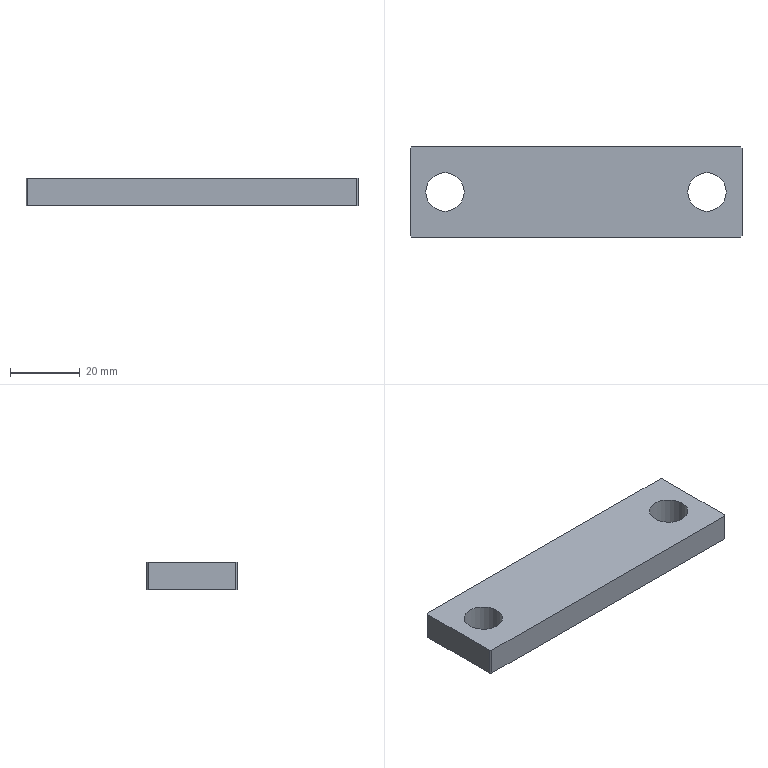Part | NX | 1 solid | 12 faces | box 95 x 26 x 8 mm | volume 18235 mm3 | plane 10 | cylinder 2 | commonest cylinder face diameters 11 x2
STEP:
#1=CARTESIAN_POINT('',(-47.5,12.5,0.));
#2=VERTEX_POINT('',#1);
#3=CARTESIAN_POINT('',(-47.5,-12.5,0.));
#4=VERTEX_POINT('',#3);
#5=CARTESIAN_POINT('',(-47.5,13.,0.));
#6=DIRECTION('',(0.,-1.,0.));
#7=VECTOR('',#6,1000.);
#8=LINE('',#5,#7);
#9=EDGE_CURVE('',#2,#4,#8,.T.);
#10=ORIENTED_EDGE('',*,*,#9,.T.);
#11=CARTESIAN_POINT('',(-47.5,-12.5,8.));
#12=VERTEX_POINT('',#11);
#13=CARTESIAN_POINT('',(-47.5,-12.5,8.));
#14=DIRECTION('',(0.,0.,1.));
#15=VECTOR('',#14,1000.);
#16=LINE('',#13,#15);
#17=EDGE_CURVE('',#4,#12,#16,.T.);
#18=ORIENTED_EDGE('',*,*,#17,.T.);
#19=CARTESIAN_POINT('',(-47.5,12.5,8.));
#20=VERTEX_POINT('',#19);
#21=CARTESIAN_POINT('',(-47.5,13.,8.));
#22=DIRECTION('',(0.,-1.,0.));
#23=VECTOR('',#22,1000.);
#24=LINE('',#21,#23);
#25=EDGE_CURVE('',#20,#12,#24,.T.);
#26=ORIENTED_EDGE('',*,*,#25,.F.);
#27=CARTESIAN_POINT('',(-47.5,12.5,8.));
#28=DIRECTION('',(0.,0.,-1.));
#29=VECTOR('',#28,1000.);
#30=LINE('',#27,#29);
#31=EDGE_CURVE('',#20,#2,#30,.T.);
#32=ORIENTED_EDGE('',*,*,#31,.T.);
#33=EDGE_LOOP('',(#10,#18,#26,#32));
#34=FACE_BOUND('',#33,.T.);
#35=CARTESIAN_POINT('',(-47.5,13.,8.));
#36=DIRECTION('',(1.,0.,0.));
#37=DIRECTION('',(0.,1.,0.));
#38=AXIS2_PLACEMENT_3D('',#35,#36,#37);
#39=PLANE('',#38);
#40=ADVANCED_FACE('',(#34),#39,.F.);
#41=CARTESIAN_POINT('',(-47.,-13.,0.));
#42=VERTEX_POINT('',#41);
#43=CARTESIAN_POINT('',(47.,-13.,0.));
#44=VERTEX_POINT('',#43);
#45=CARTESIAN_POINT('',(47.5,-13.,0.));
#46=DIRECTION('',(1.,0.,0.));
#47=VECTOR('',#46,1000.);
#48=LINE('',#45,#47);
#49=EDGE_CURVE('',#42,#44,#48,.T.);
#50=ORIENTED_EDGE('',*,*,#49,.T.);
#51=CARTESIAN_POINT('',(47.,-13.,8.));
#52=VERTEX_POINT('',#51);
#53=CARTESIAN_POINT('',(47.,-13.,8.));
#54=DIRECTION('',(0.,0.,1.));
#55=VECTOR('',#54,1000.);
#56=LINE('',#53,#55);
#57=EDGE_CURVE('',#44,#52,#56,.T.);
#58=ORIENTED_EDGE('',*,*,#57,.T.);
#59=CARTESIAN_POINT('',(-47.,-13.,8.));
#60=VERTEX_POINT('',#59);
#61=CARTESIAN_POINT('',(47.5,-13.,8.));
#62=DIRECTION('',(1.,0.,0.));
#63=VECTOR('',#62,1000.);
#64=LINE('',#61,#63);
#65=EDGE_CURVE('',#60,#52,#64,.T.);
#66=ORIENTED_EDGE('',*,*,#65,.F.);
#67=CARTESIAN_POINT('',(-47.,-13.,8.));
#68=DIRECTION('',(0.,0.,-1.));
#69=VECTOR('',#68,1000.);
#70=LINE('',#67,#69);
#71=EDGE_CURVE('',#60,#42,#70,.T.);
#72=ORIENTED_EDGE('',*,*,#71,.T.);
#73=EDGE_LOOP('',(#50,#58,#66,#72));
#74=FACE_BOUND('',#73,.T.);
#75=CARTESIAN_POINT('',(47.5,-13.,8.));
#76=DIRECTION('',(0.,1.,0.));
#77=DIRECTION('',(-1.,0.,0.));
#78=AXIS2_PLACEMENT_3D('',#75,#76,#77);
#79=PLANE('',#78);
#80=ADVANCED_FACE('',(#74),#79,.F.);
#81=CARTESIAN_POINT('',(47.5,-12.5,8.));
#82=VERTEX_POINT('',#81);
#83=CARTESIAN_POINT('',(47.5,12.5,8.));
#84=VERTEX_POINT('',#83);
#85=CARTESIAN_POINT('',(47.5,13.,8.));
#86=DIRECTION('',(0.,1.,0.));
#87=VECTOR('',#86,1000.);
#88=LINE('',#85,#87);
#89=EDGE_CURVE('',#82,#84,#88,.T.);
#90=ORIENTED_EDGE('',*,*,#89,.F.);
#91=CARTESIAN_POINT('',(47.5,-12.5,0.));
#92=VERTEX_POINT('',#91);
#93=CARTESIAN_POINT('',(47.5,-12.5,8.));
#94=DIRECTION('',(0.,0.,-1.));
#95=VECTOR('',#94,1000.);
#96=LINE('',#93,#95);
#97=EDGE_CURVE('',#82,#92,#96,.T.);
#98=ORIENTED_EDGE('',*,*,#97,.T.);
#99=CARTESIAN_POINT('',(47.5,12.5,0.));
#100=VERTEX_POINT('',#99);
#101=CARTESIAN_POINT('',(47.5,13.,0.));
#102=DIRECTION('',(0.,1.,0.));
#103=VECTOR('',#102,1000.);
#104=LINE('',#101,#103);
#105=EDGE_CURVE('',#92,#100,#104,.T.);
#106=ORIENTED_EDGE('',*,*,#105,.T.);
#107=CARTESIAN_POINT('',(47.5,12.5,8.));
#108=DIRECTION('',(0.,0.,1.));
#109=VECTOR('',#108,1000.);
#110=LINE('',#107,#109);
#111=EDGE_CURVE('',#100,#84,#110,.T.);
#112=ORIENTED_EDGE('',*,*,#111,.T.);
#113=EDGE_LOOP('',(#90,#98,#106,#112));
#114=FACE_BOUND('',#113,.T.);
#115=CARTESIAN_POINT('',(47.5,13.,8.));
#116=DIRECTION('',(-1.,0.,0.));
#117=DIRECTION('',(0.,-1.,0.));
#118=AXIS2_PLACEMENT_3D('',#115,#116,#117);
#119=PLANE('',#118);
#120=ADVANCED_FACE('',(#114),#119,.F.);
#121=CARTESIAN_POINT('',(47.,13.,8.));
#122=VERTEX_POINT('',#121);
#123=CARTESIAN_POINT('',(-47.,13.,8.));
#124=VERTEX_POINT('',#123);
#125=CARTESIAN_POINT('',(47.5,13.,8.));
#126=DIRECTION('',(-1.,0.,0.));
#127=VECTOR('',#126,1000.);
#128=LINE('',#125,#127);
#129=EDGE_CURVE('',#122,#124,#128,.T.);
#130=ORIENTED_EDGE('',*,*,#129,.F.);
#131=CARTESIAN_POINT('',(47.,13.,0.));
#132=VERTEX_POINT('',#131);
#133=CARTESIAN_POINT('',(47.,13.,8.));
#134=DIRECTION('',(0.,0.,-1.));
#135=VECTOR('',#134,1000.);
#136=LINE('',#133,#135);
#137=EDGE_CURVE('',#122,#132,#136,.T.);
#138=ORIENTED_EDGE('',*,*,#137,.T.);
#139=CARTESIAN_POINT('',(-47.,13.,0.));
#140=VERTEX_POINT('',#139);
#141=CARTESIAN_POINT('',(47.5,13.,0.));
#142=DIRECTION('',(-1.,0.,0.));
#143=VECTOR('',#142,1000.);
#144=LINE('',#141,#143);
#145=EDGE_CURVE('',#132,#140,#144,.T.);
#146=ORIENTED_EDGE('',*,*,#145,.T.);
#147=CARTESIAN_POINT('',(-47.,13.,8.));
#148=DIRECTION('',(0.,0.,1.));
#149=VECTOR('',#148,1000.);
#150=LINE('',#147,#149);
#151=EDGE_CURVE('',#140,#124,#150,.T.);
#152=ORIENTED_EDGE('',*,*,#151,.T.);
#153=EDGE_LOOP('',(#130,#138,#146,#152));
#154=FACE_BOUND('',#153,.T.);
#155=CARTESIAN_POINT('',(47.5,13.,8.));
#156=DIRECTION('',(0.,-1.,0.));
#157=DIRECTION('',(1.,0.,0.));
#158=AXIS2_PLACEMENT_3D('',#155,#156,#157);
#159=PLANE('',#158);
#160=ADVANCED_FACE('',(#154),#159,.F.);
#161=CARTESIAN_POINT('',(-43.,0.,8.));
#162=VERTEX_POINT('',#161);
#163=CARTESIAN_POINT('',(-37.5,0.,8.));
#164=DIRECTION('',(0.,0.,-1.));
#165=DIRECTION('',(-1.,0.,0.));
#166=AXIS2_PLACEMENT_3D('',#163,#164,#165);
#167=CIRCLE('',#166,5.5);
#168=EDGE_CURVE('',#162,#162,#167,.T.);
#169=ORIENTED_EDGE('',*,*,#168,.T.);
#170=EDGE_LOOP('',(#169));
#171=FACE_BOUND('',#170,.T.);
#172=CARTESIAN_POINT('',(32.,0.,8.));
#173=VERTEX_POINT('',#172);
#174=CARTESIAN_POINT('',(37.5,0.,8.));
#175=DIRECTION('',(0.,0.,-1.));
#176=DIRECTION('',(-1.,0.,0.));
#177=AXIS2_PLACEMENT_3D('',#174,#175,#176);
#178=CIRCLE('',#177,5.5);
#179=EDGE_CURVE('',#173,#173,#178,.T.);
#180=ORIENTED_EDGE('',*,*,#179,.T.);
#181=EDGE_LOOP('',(#180));
#182=FACE_BOUND('',#181,.T.);
#183=ORIENTED_EDGE('',*,*,#65,.T.);
#184=CARTESIAN_POINT('',(47.5,-12.5,8.));
#185=DIRECTION('',(-0.7071,-0.7071,0.));
#186=VECTOR('',#185,1000.);
#187=LINE('',#184,#186);
#188=EDGE_CURVE('',#52,#82,#187,.F.);
#189=ORIENTED_EDGE('',*,*,#188,.T.);
#190=ORIENTED_EDGE('',*,*,#89,.T.);
#191=CARTESIAN_POINT('',(47.,13.,8.));
#192=DIRECTION('',(0.7071,-0.7071,0.));
#193=VECTOR('',#192,1000.);
#194=LINE('',#191,#193);
#195=EDGE_CURVE('',#84,#122,#194,.F.);
#196=ORIENTED_EDGE('',*,*,#195,.T.);
#197=ORIENTED_EDGE('',*,*,#129,.T.);
#198=CARTESIAN_POINT('',(-47.5,12.5,8.));
#199=DIRECTION('',(0.7071,0.7071,0.));
#200=VECTOR('',#199,1000.);
#201=LINE('',#198,#200);
#202=EDGE_CURVE('',#124,#20,#201,.F.);
#203=ORIENTED_EDGE('',*,*,#202,.T.);
#204=ORIENTED_EDGE('',*,*,#25,.T.);
#205=CARTESIAN_POINT('',(-47.,-13.,8.));
#206=DIRECTION('',(-0.7071,0.7071,0.));
#207=VECTOR('',#206,1000.);
#208=LINE('',#205,#207);
#209=EDGE_CURVE('',#12,#60,#208,.F.);
#210=ORIENTED_EDGE('',*,*,#209,.T.);
#211=EDGE_LOOP('',(#183,#189,#190,#196,#197,#203,#204,#210));
#212=FACE_BOUND('',#211,.T.);
#213=CARTESIAN_POINT('',(0.,0.,8.));
#214=DIRECTION('',(0.,0.,-1.));
#215=DIRECTION('',(-1.,0.,0.));
#216=AXIS2_PLACEMENT_3D('',#213,#214,#215);
#217=PLANE('',#216);
#218=ADVANCED_FACE('',(#171,#182,#212),#217,.F.);
#219=CARTESIAN_POINT('',(-43.,0.,0.));
#220=VERTEX_POINT('',#219);
#221=CARTESIAN_POINT('',(-37.5,0.,0.));
#222=DIRECTION('',(0.,0.,-1.));
#223=DIRECTION('',(-1.,0.,0.));
#224=AXIS2_PLACEMENT_3D('',#221,#222,#223);
#225=CIRCLE('',#224,5.5);
#226=EDGE_CURVE('',#220,#220,#225,.T.);
#227=ORIENTED_EDGE('',*,*,#226,.F.);
#228=EDGE_LOOP('',(#227));
#229=FACE_BOUND('',#228,.T.);
#230=CARTESIAN_POINT('',(32.,0.,0.));
#231=VERTEX_POINT('',#230);
#232=CARTESIAN_POINT('',(37.5,0.,0.));
#233=DIRECTION('',(0.,0.,-1.));
#234=DIRECTION('',(-1.,0.,0.));
#235=AXIS2_PLACEMENT_3D('',#232,#233,#234);
#236=CIRCLE('',#235,5.5);
#237=EDGE_CURVE('',#231,#231,#236,.T.);
#238=ORIENTED_EDGE('',*,*,#237,.F.);
#239=EDGE_LOOP('',(#238));
#240=FACE_BOUND('',#239,.T.);
#241=ORIENTED_EDGE('',*,*,#105,.F.);
#242=CARTESIAN_POINT('',(30.,-30.,0.));
#243=DIRECTION('',(0.7071,0.7071,0.));
#244=VECTOR('',#243,1000.);
#245=LINE('',#242,#244);
#246=EDGE_CURVE('',#92,#44,#245,.F.);
#247=ORIENTED_EDGE('',*,*,#246,.T.);
#248=ORIENTED_EDGE('',*,*,#49,.F.);
#249=CARTESIAN_POINT('',(-30.,-30.,0.));
#250=DIRECTION('',(0.7071,-0.7071,0.));
#251=VECTOR('',#250,1000.);
#252=LINE('',#249,#251);
#253=EDGE_CURVE('',#42,#4,#252,.F.);
#254=ORIENTED_EDGE('',*,*,#253,.T.);
#255=ORIENTED_EDGE('',*,*,#9,.F.);
#256=CARTESIAN_POINT('',(-30.,30.,0.));
#257=DIRECTION('',(-0.7071,-0.7071,0.));
#258=VECTOR('',#257,1000.);
#259=LINE('',#256,#258);
#260=EDGE_CURVE('',#2,#140,#259,.F.);
#261=ORIENTED_EDGE('',*,*,#260,.T.);
#262=ORIENTED_EDGE('',*,*,#145,.F.);
#263=CARTESIAN_POINT('',(30.,30.,0.));
#264=DIRECTION('',(-0.7071,0.7071,0.));
#265=VECTOR('',#264,1000.);
#266=LINE('',#263,#265);
#267=EDGE_CURVE('',#132,#100,#266,.F.);
#268=ORIENTED_EDGE('',*,*,#267,.T.);
#269=EDGE_LOOP('',(#241,#247,#248,#254,#255,#261,#262,#268));
#270=FACE_BOUND('',#269,.T.);
#271=CARTESIAN_POINT('',(0.,0.,0.));
#272=DIRECTION('',(0.,0.,-1.));
#273=DIRECTION('',(-1.,0.,0.));
#274=AXIS2_PLACEMENT_3D('',#271,#272,#273);
#275=PLANE('',#274);
#276=ADVANCED_FACE('',(#229,#240,#270),#275,.T.);
#277=ORIENTED_EDGE('',*,*,#179,.F.);
#278=EDGE_LOOP('',(#277));
#279=FACE_BOUND('',#278,.T.);
#280=ORIENTED_EDGE('',*,*,#237,.T.);
#281=EDGE_LOOP('',(#280));
#282=FACE_BOUND('',#281,.T.);
#283=CARTESIAN_POINT('',(37.5,0.,0.));
#284=DIRECTION('',(0.,0.,-1.));
#285=DIRECTION('',(-1.,0.,0.));
#286=AXIS2_PLACEMENT_3D('',#283,#284,#285);
#287=CYLINDRICAL_SURFACE('',#286,5.5);
#288=ADVANCED_FACE('',(#279,#282),#287,.F.);
#289=ORIENTED_EDGE('',*,*,#168,.F.);
#290=EDGE_LOOP('',(#289));
#291=FACE_BOUND('',#290,.T.);
#292=ORIENTED_EDGE('',*,*,#226,.T.);
#293=EDGE_LOOP('',(#292));
#294=FACE_BOUND('',#293,.T.);
#295=CARTESIAN_POINT('',(-37.5,0.,0.));
#296=DIRECTION('',(0.,0.,-1.));
#297=DIRECTION('',(-1.,0.,0.));
#298=AXIS2_PLACEMENT_3D('',#295,#296,#297);
#299=CYLINDRICAL_SURFACE('',#298,5.5);
#300=ADVANCED_FACE('',(#291,#294),#299,.F.);
#301=ORIENTED_EDGE('',*,*,#188,.F.);
#302=ORIENTED_EDGE('',*,*,#57,.F.);
#303=ORIENTED_EDGE('',*,*,#246,.F.);
#304=ORIENTED_EDGE('',*,*,#97,.F.);
#305=EDGE_LOOP('',(#301,#302,#303,#304));
#306=FACE_BOUND('',#305,.T.);
#307=CARTESIAN_POINT('',(47.5,-12.5,8.));
#308=DIRECTION('',(-0.7071,0.7071,0.));
#309=DIRECTION('',(0.,0.,-1.));
#310=AXIS2_PLACEMENT_3D('',#307,#308,#309);
#311=PLANE('',#310);
#312=ADVANCED_FACE('',(#306),#311,.F.);
#313=ORIENTED_EDGE('',*,*,#195,.F.);
#314=ORIENTED_EDGE('',*,*,#111,.F.);
#315=ORIENTED_EDGE('',*,*,#267,.F.);
#316=ORIENTED_EDGE('',*,*,#137,.F.);
#317=EDGE_LOOP('',(#313,#314,#315,#316));
#318=FACE_BOUND('',#317,.T.);
#319=CARTESIAN_POINT('',(47.,13.,8.));
#320=DIRECTION('',(-0.7071,-0.7071,0.));
#321=DIRECTION('',(0.,0.,-1.));
#322=AXIS2_PLACEMENT_3D('',#319,#320,#321);
#323=PLANE('',#322);
#324=ADVANCED_FACE('',(#318),#323,.F.);
#325=ORIENTED_EDGE('',*,*,#209,.F.);
#326=ORIENTED_EDGE('',*,*,#17,.F.);
#327=ORIENTED_EDGE('',*,*,#253,.F.);
#328=ORIENTED_EDGE('',*,*,#71,.F.);
#329=EDGE_LOOP('',(#325,#326,#327,#328));
#330=FACE_BOUND('',#329,.T.);
#331=CARTESIAN_POINT('',(-47.,-13.,8.));
#332=DIRECTION('',(0.7071,0.7071,0.));
#333=DIRECTION('',(0.,0.,-1.));
#334=AXIS2_PLACEMENT_3D('',#331,#332,#333);
#335=PLANE('',#334);
#336=ADVANCED_FACE('',(#330),#335,.F.);
#337=ORIENTED_EDGE('',*,*,#202,.F.);
#338=ORIENTED_EDGE('',*,*,#151,.F.);
#339=ORIENTED_EDGE('',*,*,#260,.F.);
#340=ORIENTED_EDGE('',*,*,#31,.F.);
#341=EDGE_LOOP('',(#337,#338,#339,#340));
#342=FACE_BOUND('',#341,.T.);
#343=CARTESIAN_POINT('',(-47.5,12.5,8.));
#344=DIRECTION('',(0.7071,-0.7071,0.));
#345=DIRECTION('',(0.,0.,-1.));
#346=AXIS2_PLACEMENT_3D('',#343,#344,#345);
#347=PLANE('',#346);
#348=ADVANCED_FACE('',(#342),#347,.F.);
#349=CLOSED_SHELL('',(#40,#80,#120,#160,#218,#276,#288,#300,#312,#324,#336,#348));
#350=MANIFOLD_SOLID_BREP('',#349);
#351=(LENGTH_UNIT()NAMED_UNIT(*)SI_UNIT(.MILLI.,.METRE.));
#352=UNCERTAINTY_MEASURE_WITH_UNIT(LENGTH_MEASURE(0.00001),#351,'','');
#353=(NAMED_UNIT(*)PLANE_ANGLE_UNIT()SI_UNIT($,.RADIAN.));
#354=(NAMED_UNIT(*)SI_UNIT($,.STERADIAN.)SOLID_ANGLE_UNIT());
#355=(GEOMETRIC_REPRESENTATION_CONTEXT(3)GLOBAL_UNCERTAINTY_ASSIGNED_CONTEXT((#352))GLOBAL_UNIT_ASSIGNED_CONTEXT((#351,#353,#354))REPRESENTATION_CONTEXT('',''));
#356=ADVANCED_BREP_SHAPE_REPRESENTATION('',(#350),#355);